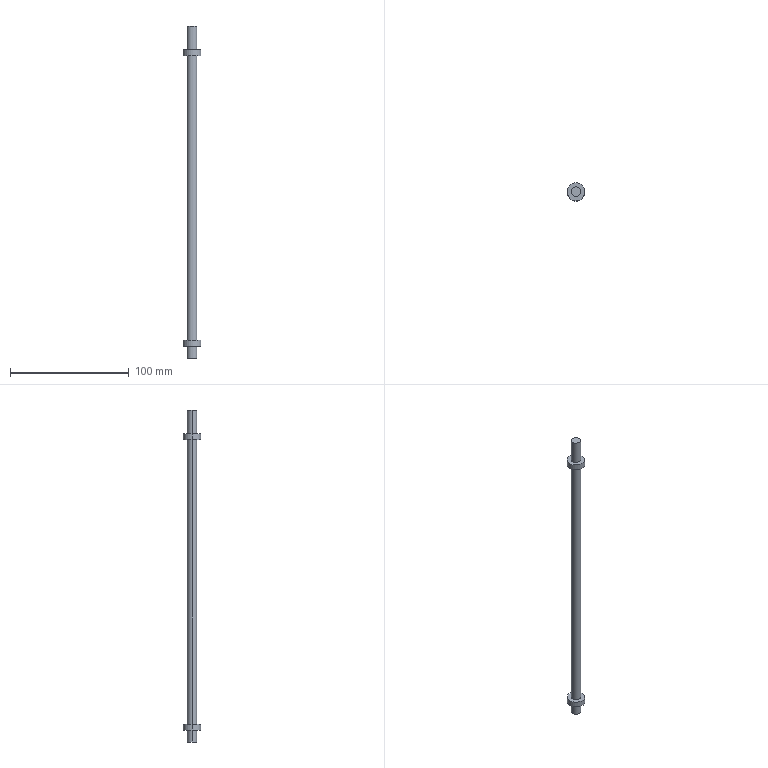Part | SolidWorks | features ICE 2, Extrusion 1 | 1 solid | 16 faces | box 15 x 15 x 280 mm | volume 15339 mm3 | cylinder 10 | plane 6 | commonest cylinder face diameters 8 x6 15 x4
STEP:
#1=CARTESIAN_POINT('',(-4.,0.,-130.));
#2=VERTEX_POINT('',#1);
#3=CARTESIAN_POINT('',(4.,0.,-130.));
#4=VERTEX_POINT('',#3);
#5=CARTESIAN_POINT('',(0.,0.,-130.));
#6=DIRECTION('',(0.,0.,-1.));
#7=DIRECTION('',(-1.,0.,0.));
#8=AXIS2_PLACEMENT_3D('',#5,#6,#7);
#9=CIRCLE('',#8,4.);
#10=EDGE_CURVE('',#2,#4,#9,.T.);
#11=ORIENTED_EDGE('',*,*,#10,.T.);
#12=CARTESIAN_POINT('',(4.,0.,-140.));
#13=VERTEX_POINT('',#12);
#14=CARTESIAN_POINT('',(4.,0.,140.));
#15=DIRECTION('',(0.,0.,-1.));
#16=VECTOR('',#15,1000.);
#17=LINE('',#14,#16);
#18=EDGE_CURVE('',#4,#13,#17,.T.);
#19=ORIENTED_EDGE('',*,*,#18,.T.);
#20=CARTESIAN_POINT('',(-4.,0.,-140.));
#21=VERTEX_POINT('',#20);
#22=CARTESIAN_POINT('',(0.,0.,-140.));
#23=DIRECTION('',(0.,0.,1.));
#24=DIRECTION('',(1.,0.,0.));
#25=AXIS2_PLACEMENT_3D('',#22,#23,#24);
#26=CIRCLE('',#25,4.);
#27=EDGE_CURVE('',#13,#21,#26,.T.);
#28=ORIENTED_EDGE('',*,*,#27,.T.);
#29=CARTESIAN_POINT('',(-4.,0.,140.));
#30=DIRECTION('',(0.,0.,-1.));
#31=VECTOR('',#30,1000.);
#32=LINE('',#29,#31);
#33=EDGE_CURVE('',#2,#21,#32,.T.);
#34=ORIENTED_EDGE('',*,*,#33,.F.);
#35=EDGE_LOOP('',(#11,#19,#28,#34));
#36=FACE_OUTER_BOUND('',#35,.T.);
#37=CARTESIAN_POINT('',(0.,0.,140.));
#38=DIRECTION('',(0.,0.,-1.));
#39=DIRECTION('',(-1.,0.,0.));
#40=AXIS2_PLACEMENT_3D('',#37,#38,#39);
#41=CYLINDRICAL_SURFACE('',#40,4.);
#42=ADVANCED_FACE('',(#36),#41,.T.);
#43=CARTESIAN_POINT('',(-7.5,0.,-125.));
#44=VERTEX_POINT('',#43);
#45=CARTESIAN_POINT('',(7.5,0.,-125.));
#46=VERTEX_POINT('',#45);
#47=CARTESIAN_POINT('',(0.,0.,-125.));
#48=DIRECTION('',(0.,0.,-1.));
#49=DIRECTION('',(-1.,0.,0.));
#50=AXIS2_PLACEMENT_3D('',#47,#48,#49);
#51=CIRCLE('',#50,7.5);
#52=EDGE_CURVE('',#44,#46,#51,.T.);
#53=ORIENTED_EDGE('',*,*,#52,.T.);
#54=CARTESIAN_POINT('',(7.5,0.,-130.));
#55=VERTEX_POINT('',#54);
#56=CARTESIAN_POINT('',(7.5,0.,-125.));
#57=DIRECTION('',(0.,0.,-1.));
#58=VECTOR('',#57,1000.);
#59=LINE('',#56,#58);
#60=EDGE_CURVE('',#46,#55,#59,.T.);
#61=ORIENTED_EDGE('',*,*,#60,.T.);
#62=CARTESIAN_POINT('',(-7.5,0.,-130.));
#63=VERTEX_POINT('',#62);
#64=CARTESIAN_POINT('',(0.,0.,-130.));
#65=DIRECTION('',(0.,0.,-1.));
#66=DIRECTION('',(-1.,0.,0.));
#67=AXIS2_PLACEMENT_3D('',#64,#65,#66);
#68=CIRCLE('',#67,7.5);
#69=EDGE_CURVE('',#63,#55,#68,.T.);
#70=ORIENTED_EDGE('',*,*,#69,.F.);
#71=CARTESIAN_POINT('',(-7.5,0.,-125.));
#72=DIRECTION('',(0.,0.,-1.));
#73=VECTOR('',#72,1000.);
#74=LINE('',#71,#73);
#75=EDGE_CURVE('',#44,#63,#74,.T.);
#76=ORIENTED_EDGE('',*,*,#75,.F.);
#77=EDGE_LOOP('',(#53,#61,#70,#76));
#78=FACE_OUTER_BOUND('',#77,.T.);
#79=CARTESIAN_POINT('',(0.,0.,-125.));
#80=DIRECTION('',(0.,0.,-1.));
#81=DIRECTION('',(-1.,0.,0.));
#82=AXIS2_PLACEMENT_3D('',#79,#80,#81);
#83=CYLINDRICAL_SURFACE('',#82,7.5);
#84=ADVANCED_FACE('',(#78),#83,.T.);
#85=CARTESIAN_POINT('',(4.,0.,140.));
#86=VERTEX_POINT('',#85);
#87=CARTESIAN_POINT('',(-4.,0.,140.));
#88=VERTEX_POINT('',#87);
#89=CARTESIAN_POINT('',(0.,0.,140.));
#90=DIRECTION('',(0.,0.,1.));
#91=DIRECTION('',(1.,0.,0.));
#92=AXIS2_PLACEMENT_3D('',#89,#90,#91);
#93=CIRCLE('',#92,4.);
#94=EDGE_CURVE('',#86,#88,#93,.T.);
#95=ORIENTED_EDGE('',*,*,#94,.F.);
#96=CARTESIAN_POINT('',(4.,0.,120.));
#97=VERTEX_POINT('',#96);
#98=CARTESIAN_POINT('',(4.,0.,140.));
#99=DIRECTION('',(0.,0.,-1.));
#100=VECTOR('',#99,1000.);
#101=LINE('',#98,#100);
#102=EDGE_CURVE('',#86,#97,#101,.T.);
#103=ORIENTED_EDGE('',*,*,#102,.T.);
#104=CARTESIAN_POINT('',(-4.,0.,120.));
#105=VERTEX_POINT('',#104);
#106=CARTESIAN_POINT('',(0.,0.,120.));
#107=DIRECTION('',(0.,0.,1.));
#108=DIRECTION('',(1.,0.,0.));
#109=AXIS2_PLACEMENT_3D('',#106,#107,#108);
#110=CIRCLE('',#109,4.);
#111=EDGE_CURVE('',#97,#105,#110,.T.);
#112=ORIENTED_EDGE('',*,*,#111,.T.);
#113=CARTESIAN_POINT('',(-4.,0.,140.));
#114=DIRECTION('',(0.,0.,-1.));
#115=VECTOR('',#114,1000.);
#116=LINE('',#113,#115);
#117=EDGE_CURVE('',#88,#105,#116,.T.);
#118=ORIENTED_EDGE('',*,*,#117,.F.);
#119=EDGE_LOOP('',(#95,#103,#112,#118));
#120=FACE_OUTER_BOUND('',#119,.T.);
#121=CARTESIAN_POINT('',(0.,0.,140.));
#122=DIRECTION('',(0.,0.,-1.));
#123=DIRECTION('',(-1.,0.,0.));
#124=AXIS2_PLACEMENT_3D('',#121,#122,#123);
#125=CYLINDRICAL_SURFACE('',#124,4.);
#126=ADVANCED_FACE('',(#120),#125,.T.);
#127=CARTESIAN_POINT('',(7.5,0.,115.));
#128=VERTEX_POINT('',#127);
#129=CARTESIAN_POINT('',(-7.5,0.,115.));
#130=VERTEX_POINT('',#129);
#131=CARTESIAN_POINT('',(0.,0.,115.));
#132=DIRECTION('',(0.,0.,1.));
#133=DIRECTION('',(1.,0.,0.));
#134=AXIS2_PLACEMENT_3D('',#131,#132,#133);
#135=CIRCLE('',#134,7.5);
#136=EDGE_CURVE('',#128,#130,#135,.T.);
#137=ORIENTED_EDGE('',*,*,#136,.T.);
#138=CARTESIAN_POINT('',(-7.5,0.,120.));
#139=VERTEX_POINT('',#138);
#140=CARTESIAN_POINT('',(-7.5,0.,115.));
#141=DIRECTION('',(0.,0.,1.));
#142=VECTOR('',#141,1000.);
#143=LINE('',#140,#142);
#144=EDGE_CURVE('',#130,#139,#143,.T.);
#145=ORIENTED_EDGE('',*,*,#144,.T.);
#146=CARTESIAN_POINT('',(7.5,0.,120.));
#147=VERTEX_POINT('',#146);
#148=CARTESIAN_POINT('',(0.,0.,120.));
#149=DIRECTION('',(0.,0.,1.));
#150=DIRECTION('',(1.,0.,0.));
#151=AXIS2_PLACEMENT_3D('',#148,#149,#150);
#152=CIRCLE('',#151,7.5);
#153=EDGE_CURVE('',#147,#139,#152,.T.);
#154=ORIENTED_EDGE('',*,*,#153,.F.);
#155=CARTESIAN_POINT('',(7.5,0.,115.));
#156=DIRECTION('',(0.,0.,1.));
#157=VECTOR('',#156,1000.);
#158=LINE('',#155,#157);
#159=EDGE_CURVE('',#128,#147,#158,.T.);
#160=ORIENTED_EDGE('',*,*,#159,.F.);
#161=EDGE_LOOP('',(#137,#145,#154,#160));
#162=FACE_OUTER_BOUND('',#161,.T.);
#163=CARTESIAN_POINT('',(0.,0.,115.));
#164=DIRECTION('',(0.,0.,1.));
#165=DIRECTION('',(1.,0.,0.));
#166=AXIS2_PLACEMENT_3D('',#163,#164,#165);
#167=CYLINDRICAL_SURFACE('',#166,7.5);
#168=ADVANCED_FACE('',(#162),#167,.T.);
#169=CARTESIAN_POINT('',(4.,0.,115.));
#170=VERTEX_POINT('',#169);
#171=CARTESIAN_POINT('',(-4.,0.,115.));
#172=VERTEX_POINT('',#171);
#173=CARTESIAN_POINT('',(0.,0.,115.));
#174=DIRECTION('',(0.,0.,1.));
#175=DIRECTION('',(1.,0.,0.));
#176=AXIS2_PLACEMENT_3D('',#173,#174,#175);
#177=CIRCLE('',#176,4.);
#178=EDGE_CURVE('',#170,#172,#177,.T.);
#179=ORIENTED_EDGE('',*,*,#178,.F.);
#180=CARTESIAN_POINT('',(4.,0.,-125.));
#181=VERTEX_POINT('',#180);
#182=CARTESIAN_POINT('',(4.,0.,140.));
#183=DIRECTION('',(0.,0.,-1.));
#184=VECTOR('',#183,1000.);
#185=LINE('',#182,#184);
#186=EDGE_CURVE('',#170,#181,#185,.T.);
#187=ORIENTED_EDGE('',*,*,#186,.T.);
#188=CARTESIAN_POINT('',(-4.,0.,-125.));
#189=VERTEX_POINT('',#188);
#190=CARTESIAN_POINT('',(0.,0.,-125.));
#191=DIRECTION('',(0.,0.,-1.));
#192=DIRECTION('',(-1.,0.,0.));
#193=AXIS2_PLACEMENT_3D('',#190,#191,#192);
#194=CIRCLE('',#193,4.);
#195=EDGE_CURVE('',#189,#181,#194,.T.);
#196=ORIENTED_EDGE('',*,*,#195,.F.);
#197=CARTESIAN_POINT('',(-4.,0.,140.));
#198=DIRECTION('',(0.,0.,-1.));
#199=VECTOR('',#198,1000.);
#200=LINE('',#197,#199);
#201=EDGE_CURVE('',#172,#189,#200,.T.);
#202=ORIENTED_EDGE('',*,*,#201,.F.);
#203=EDGE_LOOP('',(#179,#187,#196,#202));
#204=FACE_OUTER_BOUND('',#203,.T.);
#205=CARTESIAN_POINT('',(0.,0.,140.));
#206=DIRECTION('',(0.,0.,-1.));
#207=DIRECTION('',(-1.,0.,0.));
#208=AXIS2_PLACEMENT_3D('',#205,#206,#207);
#209=CYLINDRICAL_SURFACE('',#208,4.);
#210=ADVANCED_FACE('',(#204),#209,.T.);
#211=ORIENTED_EDGE('',*,*,#186,.F.);
#212=CARTESIAN_POINT('',(0.,0.,115.));
#213=DIRECTION('',(0.,0.,1.));
#214=DIRECTION('',(1.,0.,0.));
#215=AXIS2_PLACEMENT_3D('',#212,#213,#214);
#216=CIRCLE('',#215,4.);
#217=EDGE_CURVE('',#172,#170,#216,.T.);
#218=ORIENTED_EDGE('',*,*,#217,.F.);
#219=ORIENTED_EDGE('',*,*,#201,.T.);
#220=CARTESIAN_POINT('',(0.,0.,-125.));
#221=DIRECTION('',(0.,0.,-1.));
#222=DIRECTION('',(-1.,0.,0.));
#223=AXIS2_PLACEMENT_3D('',#220,#221,#222);
#224=CIRCLE('',#223,4.);
#225=EDGE_CURVE('',#181,#189,#224,.T.);
#226=ORIENTED_EDGE('',*,*,#225,.F.);
#227=EDGE_LOOP('',(#211,#218,#219,#226));
#228=FACE_OUTER_BOUND('',#227,.T.);
#229=CARTESIAN_POINT('',(0.,0.,140.));
#230=DIRECTION('',(0.,0.,-1.));
#231=DIRECTION('',(-1.,0.,0.));
#232=AXIS2_PLACEMENT_3D('',#229,#230,#231);
#233=CYLINDRICAL_SURFACE('',#232,4.);
#234=ADVANCED_FACE('',(#228),#233,.T.);
#235=ORIENTED_EDGE('',*,*,#144,.F.);
#236=CARTESIAN_POINT('',(0.,0.,115.));
#237=DIRECTION('',(0.,0.,1.));
#238=DIRECTION('',(1.,0.,0.));
#239=AXIS2_PLACEMENT_3D('',#236,#237,#238);
#240=CIRCLE('',#239,7.5);
#241=EDGE_CURVE('',#130,#128,#240,.T.);
#242=ORIENTED_EDGE('',*,*,#241,.T.);
#243=ORIENTED_EDGE('',*,*,#159,.T.);
#244=CARTESIAN_POINT('',(0.,0.,120.));
#245=DIRECTION('',(0.,0.,1.));
#246=DIRECTION('',(1.,0.,0.));
#247=AXIS2_PLACEMENT_3D('',#244,#245,#246);
#248=CIRCLE('',#247,7.5);
#249=EDGE_CURVE('',#139,#147,#248,.T.);
#250=ORIENTED_EDGE('',*,*,#249,.F.);
#251=EDGE_LOOP('',(#235,#242,#243,#250));
#252=FACE_OUTER_BOUND('',#251,.T.);
#253=CARTESIAN_POINT('',(0.,0.,115.));
#254=DIRECTION('',(0.,0.,1.));
#255=DIRECTION('',(1.,0.,0.));
#256=AXIS2_PLACEMENT_3D('',#253,#254,#255);
#257=CYLINDRICAL_SURFACE('',#256,7.5);
#258=ADVANCED_FACE('',(#252),#257,.T.);
#259=ORIENTED_EDGE('',*,*,#217,.T.);
#260=ORIENTED_EDGE('',*,*,#178,.T.);
#261=EDGE_LOOP('',(#259,#260));
#262=FACE_BOUND('',#261,.T.);
#263=ORIENTED_EDGE('',*,*,#136,.F.);
#264=ORIENTED_EDGE('',*,*,#241,.F.);
#265=EDGE_LOOP('',(#263,#264));
#266=FACE_OUTER_BOUND('',#265,.T.);
#267=CARTESIAN_POINT('',(0.,0.,115.));
#268=DIRECTION('',(0.,0.,1.));
#269=DIRECTION('',(1.,0.,0.));
#270=AXIS2_PLACEMENT_3D('',#267,#268,#269);
#271=PLANE('',#270);
#272=ADVANCED_FACE('',(#262,#266),#271,.F.);
#273=CARTESIAN_POINT('',(0.,0.,120.));
#274=DIRECTION('',(0.,0.,1.));
#275=DIRECTION('',(1.,0.,0.));
#276=AXIS2_PLACEMENT_3D('',#273,#274,#275);
#277=CIRCLE('',#276,4.);
#278=EDGE_CURVE('',#105,#97,#277,.T.);
#279=ORIENTED_EDGE('',*,*,#278,.F.);
#280=ORIENTED_EDGE('',*,*,#111,.F.);
#281=EDGE_LOOP('',(#279,#280));
#282=FACE_BOUND('',#281,.T.);
#283=ORIENTED_EDGE('',*,*,#153,.T.);
#284=ORIENTED_EDGE('',*,*,#249,.T.);
#285=EDGE_LOOP('',(#283,#284));
#286=FACE_OUTER_BOUND('',#285,.T.);
#287=CARTESIAN_POINT('',(0.,0.,120.));
#288=DIRECTION('',(0.,0.,1.));
#289=DIRECTION('',(1.,0.,0.));
#290=AXIS2_PLACEMENT_3D('',#287,#288,#289);
#291=PLANE('',#290);
#292=ADVANCED_FACE('',(#282,#286),#291,.T.);
#293=CARTESIAN_POINT('',(0.,0.,140.));
#294=DIRECTION('',(0.,0.,1.));
#295=DIRECTION('',(1.,0.,0.));
#296=AXIS2_PLACEMENT_3D('',#293,#294,#295);
#297=CIRCLE('',#296,4.);
#298=EDGE_CURVE('',#88,#86,#297,.T.);
#299=ORIENTED_EDGE('',*,*,#298,.T.);
#300=ORIENTED_EDGE('',*,*,#94,.T.);
#301=EDGE_LOOP('',(#299,#300));
#302=FACE_OUTER_BOUND('',#301,.T.);
#303=CARTESIAN_POINT('',(0.,0.,140.));
#304=DIRECTION('',(0.,0.,1.));
#305=DIRECTION('',(1.,0.,0.));
#306=AXIS2_PLACEMENT_3D('',#303,#304,#305);
#307=PLANE('',#306);
#308=ADVANCED_FACE('',(#302),#307,.T.);
#309=ORIENTED_EDGE('',*,*,#102,.F.);
#310=ORIENTED_EDGE('',*,*,#298,.F.);
#311=ORIENTED_EDGE('',*,*,#117,.T.);
#312=ORIENTED_EDGE('',*,*,#278,.T.);
#313=EDGE_LOOP('',(#309,#310,#311,#312));
#314=FACE_OUTER_BOUND('',#313,.T.);
#315=CARTESIAN_POINT('',(0.,0.,140.));
#316=DIRECTION('',(0.,0.,-1.));
#317=DIRECTION('',(-1.,0.,0.));
#318=AXIS2_PLACEMENT_3D('',#315,#316,#317);
#319=CYLINDRICAL_SURFACE('',#318,4.);
#320=ADVANCED_FACE('',(#314),#319,.T.);
#321=ORIENTED_EDGE('',*,*,#60,.F.);
#322=CARTESIAN_POINT('',(0.,0.,-125.));
#323=DIRECTION('',(0.,0.,-1.));
#324=DIRECTION('',(-1.,0.,0.));
#325=AXIS2_PLACEMENT_3D('',#322,#323,#324);
#326=CIRCLE('',#325,7.5);
#327=EDGE_CURVE('',#46,#44,#326,.T.);
#328=ORIENTED_EDGE('',*,*,#327,.T.);
#329=ORIENTED_EDGE('',*,*,#75,.T.);
#330=CARTESIAN_POINT('',(0.,0.,-130.));
#331=DIRECTION('',(0.,0.,-1.));
#332=DIRECTION('',(-1.,0.,0.));
#333=AXIS2_PLACEMENT_3D('',#330,#331,#332);
#334=CIRCLE('',#333,7.5);
#335=EDGE_CURVE('',#55,#63,#334,.T.);
#336=ORIENTED_EDGE('',*,*,#335,.F.);
#337=EDGE_LOOP('',(#321,#328,#329,#336));
#338=FACE_OUTER_BOUND('',#337,.T.);
#339=CARTESIAN_POINT('',(0.,0.,-125.));
#340=DIRECTION('',(0.,0.,-1.));
#341=DIRECTION('',(-1.,0.,0.));
#342=AXIS2_PLACEMENT_3D('',#339,#340,#341);
#343=CYLINDRICAL_SURFACE('',#342,7.5);
#344=ADVANCED_FACE('',(#338),#343,.T.);
#345=ORIENTED_EDGE('',*,*,#195,.T.);
#346=ORIENTED_EDGE('',*,*,#225,.T.);
#347=EDGE_LOOP('',(#345,#346));
#348=FACE_BOUND('',#347,.T.);
#349=ORIENTED_EDGE('',*,*,#52,.F.);
#350=ORIENTED_EDGE('',*,*,#327,.F.);
#351=EDGE_LOOP('',(#349,#350));
#352=FACE_OUTER_BOUND('',#351,.T.);
#353=CARTESIAN_POINT('',(0.,0.,-125.));
#354=DIRECTION('',(0.,0.,-1.));
#355=DIRECTION('',(-1.,0.,0.));
#356=AXIS2_PLACEMENT_3D('',#353,#354,#355);
#357=PLANE('',#356);
#358=ADVANCED_FACE('',(#348,#352),#357,.F.);
#359=ORIENTED_EDGE('',*,*,#10,.F.);
#360=CARTESIAN_POINT('',(0.,0.,-130.));
#361=DIRECTION('',(0.,0.,-1.));
#362=DIRECTION('',(-1.,0.,0.));
#363=AXIS2_PLACEMENT_3D('',#360,#361,#362);
#364=CIRCLE('',#363,4.);
#365=EDGE_CURVE('',#4,#2,#364,.T.);
#366=ORIENTED_EDGE('',*,*,#365,.F.);
#367=EDGE_LOOP('',(#359,#366));
#368=FACE_BOUND('',#367,.T.);
#369=ORIENTED_EDGE('',*,*,#69,.T.);
#370=ORIENTED_EDGE('',*,*,#335,.T.);
#371=EDGE_LOOP('',(#369,#370));
#372=FACE_OUTER_BOUND('',#371,.T.);
#373=CARTESIAN_POINT('',(0.,0.,-130.));
#374=DIRECTION('',(0.,0.,-1.));
#375=DIRECTION('',(-1.,0.,0.));
#376=AXIS2_PLACEMENT_3D('',#373,#374,#375);
#377=PLANE('',#376);
#378=ADVANCED_FACE('',(#368,#372),#377,.T.);
#379=CARTESIAN_POINT('',(0.,0.,-140.));
#380=DIRECTION('',(0.,0.,1.));
#381=DIRECTION('',(1.,0.,0.));
#382=AXIS2_PLACEMENT_3D('',#379,#380,#381);
#383=CIRCLE('',#382,4.);
#384=EDGE_CURVE('',#21,#13,#383,.T.);
#385=ORIENTED_EDGE('',*,*,#384,.F.);
#386=ORIENTED_EDGE('',*,*,#27,.F.);
#387=EDGE_LOOP('',(#385,#386));
#388=FACE_OUTER_BOUND('',#387,.T.);
#389=CARTESIAN_POINT('',(0.,0.,-140.));
#390=DIRECTION('',(0.,0.,1.));
#391=DIRECTION('',(1.,0.,0.));
#392=AXIS2_PLACEMENT_3D('',#389,#390,#391);
#393=PLANE('',#392);
#394=ADVANCED_FACE('',(#388),#393,.F.);
#395=ORIENTED_EDGE('',*,*,#18,.F.);
#396=ORIENTED_EDGE('',*,*,#365,.T.);
#397=ORIENTED_EDGE('',*,*,#33,.T.);
#398=ORIENTED_EDGE('',*,*,#384,.T.);
#399=EDGE_LOOP('',(#395,#396,#397,#398));
#400=FACE_OUTER_BOUND('',#399,.T.);
#401=CARTESIAN_POINT('',(0.,0.,140.));
#402=DIRECTION('',(0.,0.,-1.));
#403=DIRECTION('',(-1.,0.,0.));
#404=AXIS2_PLACEMENT_3D('',#401,#402,#403);
#405=CYLINDRICAL_SURFACE('',#404,4.);
#406=ADVANCED_FACE('',(#400),#405,.T.);
#407=CLOSED_SHELL('',(#42,#84,#126,#168,#210,#234,#258,#272,#292,#308,#320,#344,#358,#378,#394,#406));
#408=MANIFOLD_SOLID_BREP('',#407);
#409=CARTESIAN_POINT('',(0.,0.,0.));
#410=DIRECTION('',(0.,0.,1.));
#411=DIRECTION('',(1.,0.,0.));
#412=AXIS2_PLACEMENT_3D('',#409,#410,#411);
#413=(LENGTH_UNIT()NAMED_UNIT(*)SI_UNIT(.MILLI.,.METRE.));
#414=UNCERTAINTY_MEASURE_WITH_UNIT(LENGTH_MEASURE(0.00001),#413,'','');
#415=(NAMED_UNIT(*)PLANE_ANGLE_UNIT()SI_UNIT($,.RADIAN.));
#416=(NAMED_UNIT(*)SI_UNIT($,.STERADIAN.)SOLID_ANGLE_UNIT());
#417=(GEOMETRIC_REPRESENTATION_CONTEXT(3)GLOBAL_UNCERTAINTY_ASSIGNED_CONTEXT((#414))GLOBAL_UNIT_ASSIGNED_CONTEXT((#413,#415,#416))REPRESENTATION_CONTEXT('',''));
#418=ADVANCED_BREP_SHAPE_REPRESENTATION('',(#408,#412),#417);